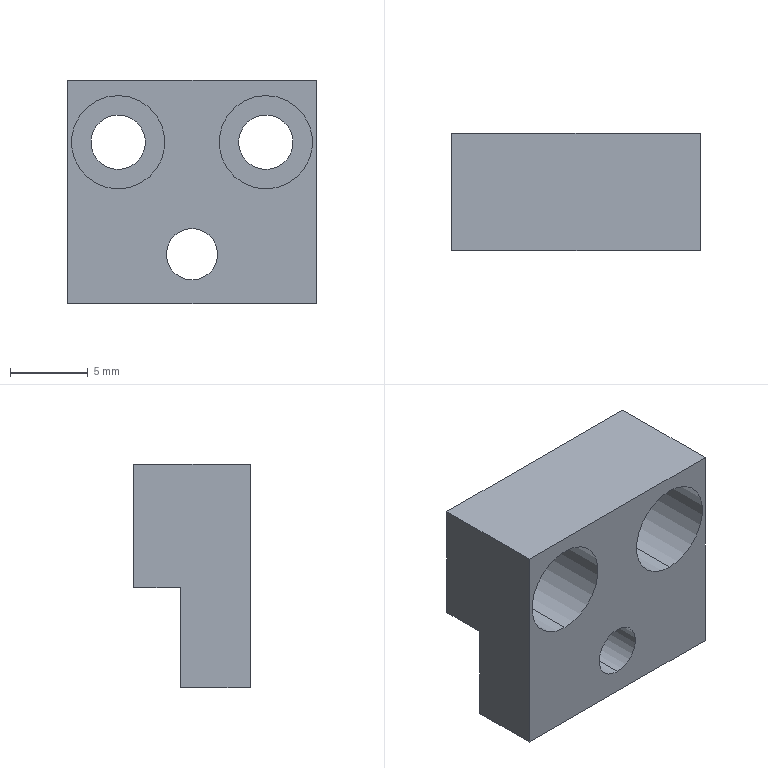Part | NX | 1 solid | 20 faces | box 16 x 7.5 x 14.4 mm | volume 1068 mm3 | plane 10 | cylinder 10 | commonest cylinder face diameters 3.5 x4 6 x4 3.3 x2
STEP:
#1=CARTESIAN_POINT('',(16.39,-66.129,11.453));
#2=VERTEX_POINT('',#1);
#3=CARTESIAN_POINT('',(16.39,-63.129,11.453));
#4=VERTEX_POINT('',#3);
#5=CARTESIAN_POINT('',(16.39,-59.69,11.453));
#6=DIRECTION('',(0.,1.,0.));
#7=VECTOR('',#6,1000.);
#8=LINE('',#5,#7);
#9=EDGE_CURVE('',#2,#4,#8,.T.);
#10=ORIENTED_EDGE('',*,*,#9,.F.);
#11=CARTESIAN_POINT('',(0.3897,-66.129,11.453));
#12=VERTEX_POINT('',#11);
#13=CARTESIAN_POINT('',(13.89,-66.129,11.453));
#14=DIRECTION('',(-1.,0.,0.));
#15=VECTOR('',#14,1000.);
#16=LINE('',#13,#15);
#17=EDGE_CURVE('',#2,#12,#16,.T.);
#18=ORIENTED_EDGE('',*,*,#17,.T.);
#19=CARTESIAN_POINT('',(0.3897,-63.129,11.453));
#20=VERTEX_POINT('',#19);
#21=CARTESIAN_POINT('',(0.3897,-59.69,11.453));
#22=DIRECTION('',(0.,1.,0.));
#23=VECTOR('',#22,1000.);
#24=LINE('',#21,#23);
#25=EDGE_CURVE('',#12,#20,#24,.T.);
#26=ORIENTED_EDGE('',*,*,#25,.T.);
#27=CARTESIAN_POINT('',(13.89,-63.129,11.453));
#28=DIRECTION('',(-1.,0.,0.));
#29=VECTOR('',#28,1000.);
#30=LINE('',#27,#29);
#31=EDGE_CURVE('',#4,#20,#30,.T.);
#32=ORIENTED_EDGE('',*,*,#31,.F.);
#33=EDGE_LOOP('',(#10,#18,#26,#32));
#34=FACE_BOUND('',#33,.T.);
#35=CARTESIAN_POINT('',(13.89,-66.629,11.453));
#36=DIRECTION('',(0.,0.,-1.));
#37=DIRECTION('',(0.,-1.,0.));
#38=AXIS2_PLACEMENT_3D('',#35,#36,#37);
#39=PLANE('',#38);
#40=ADVANCED_FACE('',(#34),#39,.T.);
#41=CARTESIAN_POINT('',(16.39,-66.129,5.003));
#42=VERTEX_POINT('',#41);
#43=CARTESIAN_POINT('',(16.39,-66.129,11.106));
#44=DIRECTION('',(0.,0.,-1.));
#45=VECTOR('',#44,1000.);
#46=LINE('',#43,#45);
#47=EDGE_CURVE('',#2,#42,#46,.T.);
#48=ORIENTED_EDGE('',*,*,#47,.T.);
#49=CARTESIAN_POINT('',(0.3897,-66.129,5.003));
#50=VERTEX_POINT('',#49);
#51=CARTESIAN_POINT('',(13.89,-66.129,5.003));
#52=DIRECTION('',(-1.,0.,0.));
#53=VECTOR('',#52,1000.);
#54=LINE('',#51,#53);
#55=EDGE_CURVE('',#42,#50,#54,.T.);
#56=ORIENTED_EDGE('',*,*,#55,.T.);
#57=CARTESIAN_POINT('',(0.3897,-66.129,11.106));
#58=DIRECTION('',(0.,0.,-1.));
#59=VECTOR('',#58,1000.);
#60=LINE('',#57,#59);
#61=EDGE_CURVE('',#12,#50,#60,.T.);
#62=ORIENTED_EDGE('',*,*,#61,.F.);
#63=ORIENTED_EDGE('',*,*,#17,.F.);
#64=EDGE_LOOP('',(#48,#56,#62,#63));
#65=FACE_BOUND('',#64,.T.);
#66=CARTESIAN_POINT('',(8.39,-66.129,6.553));
#67=VERTEX_POINT('',#66);
#68=CARTESIAN_POINT('',(8.39,-66.129,9.853));
#69=VERTEX_POINT('',#68);
#70=CARTESIAN_POINT('',(8.39,-66.129,8.203));
#71=DIRECTION('',(0.,-1.,0.));
#72=DIRECTION('',(0.,0.,1.));
#73=AXIS2_PLACEMENT_3D('',#70,#71,#72);
#74=CIRCLE('',#73,1.65);
#75=EDGE_CURVE('',#67,#69,#74,.T.);
#76=ORIENTED_EDGE('',*,*,#75,.T.);
#77=CARTESIAN_POINT('',(8.39,-66.129,8.203));
#78=DIRECTION('',(0.,-1.,0.));
#79=DIRECTION('',(0.,0.,1.));
#80=AXIS2_PLACEMENT_3D('',#77,#78,#79);
#81=CIRCLE('',#80,1.65);
#82=EDGE_CURVE('',#69,#67,#81,.T.);
#83=ORIENTED_EDGE('',*,*,#82,.T.);
#84=EDGE_LOOP('',(#76,#83));
#85=FACE_BOUND('',#84,.T.);
#86=CARTESIAN_POINT('',(13.89,-66.129,5.503));
#87=DIRECTION('',(0.,1.,0.));
#88=DIRECTION('',(1.,0.,0.));
#89=AXIS2_PLACEMENT_3D('',#86,#87,#88);
#90=PLANE('',#89);
#91=ADVANCED_FACE('',(#65,#85),#90,.T.);
#92=CARTESIAN_POINT('',(0.3897,-70.629,5.003));
#93=VERTEX_POINT('',#92);
#94=CARTESIAN_POINT('',(16.39,-70.629,5.003));
#95=VERTEX_POINT('',#94);
#96=CARTESIAN_POINT('',(13.89,-70.629,5.003));
#97=DIRECTION('',(1.,0.,0.));
#98=VECTOR('',#97,1000.);
#99=LINE('',#96,#98);
#100=EDGE_CURVE('',#93,#95,#99,.T.);
#101=ORIENTED_EDGE('',*,*,#100,.F.);
#102=CARTESIAN_POINT('',(0.3897,-59.69,5.003));
#103=DIRECTION('',(0.,-1.,0.));
#104=VECTOR('',#103,1000.);
#105=LINE('',#102,#104);
#106=EDGE_CURVE('',#50,#93,#105,.T.);
#107=ORIENTED_EDGE('',*,*,#106,.F.);
#108=ORIENTED_EDGE('',*,*,#55,.F.);
#109=CARTESIAN_POINT('',(16.39,-59.69,5.003));
#110=DIRECTION('',(0.,-1.,0.));
#111=VECTOR('',#110,1000.);
#112=LINE('',#109,#111);
#113=EDGE_CURVE('',#42,#95,#112,.T.);
#114=ORIENTED_EDGE('',*,*,#113,.T.);
#115=EDGE_LOOP('',(#101,#107,#108,#114));
#116=FACE_BOUND('',#115,.T.);
#117=CARTESIAN_POINT('',(13.89,-70.329,5.003));
#118=DIRECTION('',(0.,0.,-1.));
#119=DIRECTION('',(0.,-1.,0.));
#120=AXIS2_PLACEMENT_3D('',#117,#118,#119);
#121=PLANE('',#120);
#122=ADVANCED_FACE('',(#116),#121,.T.);
#123=CARTESIAN_POINT('',(16.39,-70.629,19.403));
#124=VERTEX_POINT('',#123);
#125=CARTESIAN_POINT('',(16.39,-70.629,11.106));
#126=DIRECTION('',(0.,0.,1.));
#127=VECTOR('',#126,1000.);
#128=LINE('',#125,#127);
#129=EDGE_CURVE('',#95,#124,#128,.T.);
#130=ORIENTED_EDGE('',*,*,#129,.T.);
#131=CARTESIAN_POINT('',(0.3897,-70.629,19.403));
#132=VERTEX_POINT('',#131);
#133=CARTESIAN_POINT('',(13.89,-70.629,19.403));
#134=DIRECTION('',(-1.,0.,0.));
#135=VECTOR('',#134,1000.);
#136=LINE('',#133,#135);
#137=EDGE_CURVE('',#124,#132,#136,.T.);
#138=ORIENTED_EDGE('',*,*,#137,.T.);
#139=CARTESIAN_POINT('',(0.3897,-70.629,11.106));
#140=DIRECTION('',(0.,0.,1.));
#141=VECTOR('',#140,1000.);
#142=LINE('',#139,#141);
#143=EDGE_CURVE('',#93,#132,#142,.T.);
#144=ORIENTED_EDGE('',*,*,#143,.F.);
#145=ORIENTED_EDGE('',*,*,#100,.T.);
#146=EDGE_LOOP('',(#130,#138,#144,#145));
#147=FACE_BOUND('',#146,.T.);
#148=CARTESIAN_POINT('',(3.64,-70.629,12.403));
#149=VERTEX_POINT('',#148);
#150=CARTESIAN_POINT('',(3.64,-70.629,18.403));
#151=VERTEX_POINT('',#150);
#152=CARTESIAN_POINT('',(3.64,-70.629,15.403));
#153=DIRECTION('',(0.,-1.,0.));
#154=DIRECTION('',(0.,0.,1.));
#155=AXIS2_PLACEMENT_3D('',#152,#153,#154);
#156=CIRCLE('',#155,3.);
#157=EDGE_CURVE('',#149,#151,#156,.T.);
#158=ORIENTED_EDGE('',*,*,#157,.F.);
#159=CARTESIAN_POINT('',(3.64,-70.629,15.403));
#160=DIRECTION('',(0.,-1.,0.));
#161=DIRECTION('',(0.,0.,1.));
#162=AXIS2_PLACEMENT_3D('',#159,#160,#161);
#163=CIRCLE('',#162,3.);
#164=EDGE_CURVE('',#151,#149,#163,.T.);
#165=ORIENTED_EDGE('',*,*,#164,.F.);
#166=EDGE_LOOP('',(#158,#165));
#167=FACE_BOUND('',#166,.T.);
#168=CARTESIAN_POINT('',(8.39,-70.629,6.553));
#169=VERTEX_POINT('',#168);
#170=CARTESIAN_POINT('',(8.39,-70.629,9.853));
#171=VERTEX_POINT('',#170);
#172=CARTESIAN_POINT('',(8.39,-70.629,8.203));
#173=DIRECTION('',(0.,-1.,0.));
#174=DIRECTION('',(0.,0.,1.));
#175=AXIS2_PLACEMENT_3D('',#172,#173,#174);
#176=CIRCLE('',#175,1.65);
#177=EDGE_CURVE('',#169,#171,#176,.T.);
#178=ORIENTED_EDGE('',*,*,#177,.F.);
#179=CARTESIAN_POINT('',(8.39,-70.629,8.203));
#180=DIRECTION('',(0.,-1.,0.));
#181=DIRECTION('',(0.,0.,1.));
#182=AXIS2_PLACEMENT_3D('',#179,#180,#181);
#183=CIRCLE('',#182,1.65);
#184=EDGE_CURVE('',#171,#169,#183,.T.);
#185=ORIENTED_EDGE('',*,*,#184,.F.);
#186=EDGE_LOOP('',(#178,#185));
#187=FACE_BOUND('',#186,.T.);
#188=CARTESIAN_POINT('',(13.14,-70.629,12.403));
#189=VERTEX_POINT('',#188);
#190=CARTESIAN_POINT('',(13.14,-70.629,18.403));
#191=VERTEX_POINT('',#190);
#192=CARTESIAN_POINT('',(13.14,-70.629,15.403));
#193=DIRECTION('',(0.,-1.,0.));
#194=DIRECTION('',(0.,0.,1.));
#195=AXIS2_PLACEMENT_3D('',#192,#193,#194);
#196=CIRCLE('',#195,3.);
#197=EDGE_CURVE('',#189,#191,#196,.T.);
#198=ORIENTED_EDGE('',*,*,#197,.F.);
#199=CARTESIAN_POINT('',(13.14,-70.629,15.403));
#200=DIRECTION('',(0.,-1.,0.));
#201=DIRECTION('',(0.,0.,1.));
#202=AXIS2_PLACEMENT_3D('',#199,#200,#201);
#203=CIRCLE('',#202,3.);
#204=EDGE_CURVE('',#191,#189,#203,.T.);
#205=ORIENTED_EDGE('',*,*,#204,.F.);
#206=EDGE_LOOP('',(#198,#205));
#207=FACE_BOUND('',#206,.T.);
#208=CARTESIAN_POINT('',(13.89,-70.629,20.403));
#209=DIRECTION('',(0.,-1.,0.));
#210=DIRECTION('',(-1.,0.,0.));
#211=AXIS2_PLACEMENT_3D('',#208,#209,#210);
#212=PLANE('',#211);
#213=ADVANCED_FACE('',(#147,#167,#187,#207),#212,.T.);
#214=CARTESIAN_POINT('',(16.39,-63.129,19.403));
#215=VERTEX_POINT('',#214);
#216=CARTESIAN_POINT('',(16.39,-59.69,19.403));
#217=DIRECTION('',(0.,1.,0.));
#218=VECTOR('',#217,1000.);
#219=LINE('',#216,#218);
#220=EDGE_CURVE('',#124,#215,#219,.T.);
#221=ORIENTED_EDGE('',*,*,#220,.T.);
#222=CARTESIAN_POINT('',(0.3897,-63.129,19.403));
#223=VERTEX_POINT('',#222);
#224=CARTESIAN_POINT('',(13.89,-63.129,19.403));
#225=DIRECTION('',(1.,0.,0.));
#226=VECTOR('',#225,1000.);
#227=LINE('',#224,#226);
#228=EDGE_CURVE('',#223,#215,#227,.T.);
#229=ORIENTED_EDGE('',*,*,#228,.F.);
#230=CARTESIAN_POINT('',(0.3897,-59.69,19.403));
#231=DIRECTION('',(0.,1.,0.));
#232=VECTOR('',#231,1000.);
#233=LINE('',#230,#232);
#234=EDGE_CURVE('',#132,#223,#233,.T.);
#235=ORIENTED_EDGE('',*,*,#234,.F.);
#236=ORIENTED_EDGE('',*,*,#137,.F.);
#237=EDGE_LOOP('',(#221,#229,#235,#236));
#238=FACE_BOUND('',#237,.T.);
#239=CARTESIAN_POINT('',(13.89,-63.129,19.403));
#240=DIRECTION('',(0.,0.,1.));
#241=DIRECTION('',(1.,0.,0.));
#242=AXIS2_PLACEMENT_3D('',#239,#240,#241);
#243=PLANE('',#242);
#244=ADVANCED_FACE('',(#238),#243,.T.);
#245=CARTESIAN_POINT('',(16.39,-63.129,11.106));
#246=DIRECTION('',(0.,0.,-1.));
#247=VECTOR('',#246,1000.);
#248=LINE('',#245,#247);
#249=EDGE_CURVE('',#215,#4,#248,.T.);
#250=ORIENTED_EDGE('',*,*,#249,.T.);
#251=ORIENTED_EDGE('',*,*,#31,.T.);
#252=CARTESIAN_POINT('',(0.3897,-63.129,11.106));
#253=DIRECTION('',(0.,0.,-1.));
#254=VECTOR('',#253,1000.);
#255=LINE('',#252,#254);
#256=EDGE_CURVE('',#223,#20,#255,.T.);
#257=ORIENTED_EDGE('',*,*,#256,.F.);
#258=ORIENTED_EDGE('',*,*,#228,.T.);
#259=EDGE_LOOP('',(#250,#251,#257,#258));
#260=FACE_BOUND('',#259,.T.);
#261=CARTESIAN_POINT('',(13.14,-63.129,13.653));
#262=VERTEX_POINT('',#261);
#263=CARTESIAN_POINT('',(13.14,-63.129,17.153));
#264=VERTEX_POINT('',#263);
#265=CARTESIAN_POINT('',(13.14,-63.129,15.403));
#266=DIRECTION('',(0.,-1.,0.));
#267=DIRECTION('',(0.,0.,1.));
#268=AXIS2_PLACEMENT_3D('',#265,#266,#267);
#269=CIRCLE('',#268,1.75);
#270=EDGE_CURVE('',#262,#264,#269,.T.);
#271=ORIENTED_EDGE('',*,*,#270,.T.);
#272=CARTESIAN_POINT('',(13.14,-63.129,15.403));
#273=DIRECTION('',(0.,-1.,0.));
#274=DIRECTION('',(0.,0.,1.));
#275=AXIS2_PLACEMENT_3D('',#272,#273,#274);
#276=CIRCLE('',#275,1.75);
#277=EDGE_CURVE('',#264,#262,#276,.T.);
#278=ORIENTED_EDGE('',*,*,#277,.T.);
#279=EDGE_LOOP('',(#271,#278));
#280=FACE_BOUND('',#279,.T.);
#281=CARTESIAN_POINT('',(3.64,-63.129,13.653));
#282=VERTEX_POINT('',#281);
#283=CARTESIAN_POINT('',(3.64,-63.129,17.153));
#284=VERTEX_POINT('',#283);
#285=CARTESIAN_POINT('',(3.64,-63.129,15.403));
#286=DIRECTION('',(0.,-1.,0.));
#287=DIRECTION('',(0.,0.,1.));
#288=AXIS2_PLACEMENT_3D('',#285,#286,#287);
#289=CIRCLE('',#288,1.75);
#290=EDGE_CURVE('',#282,#284,#289,.T.);
#291=ORIENTED_EDGE('',*,*,#290,.T.);
#292=CARTESIAN_POINT('',(3.64,-63.129,15.403));
#293=DIRECTION('',(0.,-1.,0.));
#294=DIRECTION('',(0.,0.,1.));
#295=AXIS2_PLACEMENT_3D('',#292,#293,#294);
#296=CIRCLE('',#295,1.75);
#297=EDGE_CURVE('',#284,#282,#296,.T.);
#298=ORIENTED_EDGE('',*,*,#297,.T.);
#299=EDGE_LOOP('',(#291,#298));
#300=FACE_BOUND('',#299,.T.);
#301=CARTESIAN_POINT('',(13.89,-63.129,11.253));
#302=DIRECTION('',(0.,1.,0.));
#303=DIRECTION('',(1.,0.,0.));
#304=AXIS2_PLACEMENT_3D('',#301,#302,#303);
#305=PLANE('',#304);
#306=ADVANCED_FACE('',(#260,#280,#300),#305,.T.);
#307=ORIENTED_EDGE('',*,*,#157,.T.);
#308=CARTESIAN_POINT('',(3.64,-66.129,18.403));
#309=VERTEX_POINT('',#308);
#310=CARTESIAN_POINT('',(3.64,-69.629,18.403));
#311=DIRECTION('',(0.,-1.,0.));
#312=VECTOR('',#311,1000.);
#313=LINE('',#310,#312);
#314=EDGE_CURVE('',#309,#151,#313,.T.);
#315=ORIENTED_EDGE('',*,*,#314,.F.);
#316=CARTESIAN_POINT('',(3.64,-66.129,12.403));
#317=VERTEX_POINT('',#316);
#318=CARTESIAN_POINT('',(3.64,-66.129,15.403));
#319=DIRECTION('',(0.,-1.,0.));
#320=DIRECTION('',(0.,0.,1.));
#321=AXIS2_PLACEMENT_3D('',#318,#319,#320);
#322=CIRCLE('',#321,3.);
#323=EDGE_CURVE('',#317,#309,#322,.T.);
#324=ORIENTED_EDGE('',*,*,#323,.F.);
#325=CARTESIAN_POINT('',(3.64,-69.629,12.403));
#326=DIRECTION('',(0.,-1.,0.));
#327=VECTOR('',#326,1000.);
#328=LINE('',#325,#327);
#329=EDGE_CURVE('',#317,#149,#328,.T.);
#330=ORIENTED_EDGE('',*,*,#329,.T.);
#331=EDGE_LOOP('',(#307,#315,#324,#330));
#332=FACE_BOUND('',#331,.T.);
#333=CARTESIAN_POINT('',(3.64,-69.629,15.403));
#334=DIRECTION('',(0.,-1.,0.));
#335=DIRECTION('',(0.,0.,1.));
#336=AXIS2_PLACEMENT_3D('',#333,#334,#335);
#337=CYLINDRICAL_SURFACE('',#336,3.);
#338=ADVANCED_FACE('',(#332),#337,.F.);
#339=ORIENTED_EDGE('',*,*,#323,.T.);
#340=CARTESIAN_POINT('',(3.64,-66.129,15.403));
#341=DIRECTION('',(0.,-1.,0.));
#342=DIRECTION('',(0.,0.,1.));
#343=AXIS2_PLACEMENT_3D('',#340,#341,#342);
#344=CIRCLE('',#343,3.);
#345=EDGE_CURVE('',#309,#317,#344,.T.);
#346=ORIENTED_EDGE('',*,*,#345,.T.);
#347=EDGE_LOOP('',(#339,#346));
#348=FACE_BOUND('',#347,.T.);
#349=CARTESIAN_POINT('',(3.64,-66.129,13.653));
#350=VERTEX_POINT('',#349);
#351=CARTESIAN_POINT('',(3.64,-66.129,17.153));
#352=VERTEX_POINT('',#351);
#353=CARTESIAN_POINT('',(3.64,-66.129,15.403));
#354=DIRECTION('',(0.,-1.,0.));
#355=DIRECTION('',(0.,0.,1.));
#356=AXIS2_PLACEMENT_3D('',#353,#354,#355);
#357=CIRCLE('',#356,1.75);
#358=EDGE_CURVE('',#350,#352,#357,.T.);
#359=ORIENTED_EDGE('',*,*,#358,.F.);
#360=CARTESIAN_POINT('',(3.64,-66.129,15.403));
#361=DIRECTION('',(0.,-1.,0.));
#362=DIRECTION('',(0.,0.,1.));
#363=AXIS2_PLACEMENT_3D('',#360,#361,#362);
#364=CIRCLE('',#363,1.75);
#365=EDGE_CURVE('',#352,#350,#364,.T.);
#366=ORIENTED_EDGE('',*,*,#365,.F.);
#367=EDGE_LOOP('',(#359,#366));
#368=FACE_BOUND('',#367,.T.);
#369=CARTESIAN_POINT('',(3.64,-66.129,15.403));
#370=DIRECTION('',(0.,-1.,0.));
#371=DIRECTION('',(-1.,0.,0.));
#372=AXIS2_PLACEMENT_3D('',#369,#370,#371);
#373=PLANE('',#372);
#374=ADVANCED_FACE('',(#348,#368),#373,.T.);
#375=ORIENTED_EDGE('',*,*,#358,.T.);
#376=CARTESIAN_POINT('',(3.64,-69.629,17.153));
#377=DIRECTION('',(0.,-1.,0.));
#378=VECTOR('',#377,1000.);
#379=LINE('',#376,#378);
#380=EDGE_CURVE('',#284,#352,#379,.T.);
#381=ORIENTED_EDGE('',*,*,#380,.F.);
#382=ORIENTED_EDGE('',*,*,#290,.F.);
#383=CARTESIAN_POINT('',(3.64,-69.629,13.653));
#384=DIRECTION('',(0.,-1.,0.));
#385=VECTOR('',#384,1000.);
#386=LINE('',#383,#385);
#387=EDGE_CURVE('',#282,#350,#386,.T.);
#388=ORIENTED_EDGE('',*,*,#387,.T.);
#389=EDGE_LOOP('',(#375,#381,#382,#388));
#390=FACE_BOUND('',#389,.T.);
#391=CARTESIAN_POINT('',(3.64,-69.629,15.403));
#392=DIRECTION('',(0.,-1.,0.));
#393=DIRECTION('',(0.,0.,1.));
#394=AXIS2_PLACEMENT_3D('',#391,#392,#393);
#395=CYLINDRICAL_SURFACE('',#394,1.75);
#396=ADVANCED_FACE('',(#390),#395,.F.);
#397=CARTESIAN_POINT('',(13.14,-66.129,13.653));
#398=VERTEX_POINT('',#397);
#399=CARTESIAN_POINT('',(13.14,-66.129,17.153));
#400=VERTEX_POINT('',#399);
#401=CARTESIAN_POINT('',(13.14,-66.129,15.403));
#402=DIRECTION('',(0.,-1.,0.));
#403=DIRECTION('',(0.,0.,1.));
#404=AXIS2_PLACEMENT_3D('',#401,#402,#403);
#405=CIRCLE('',#404,1.75);
#406=EDGE_CURVE('',#398,#400,#405,.T.);
#407=ORIENTED_EDGE('',*,*,#406,.T.);
#408=CARTESIAN_POINT('',(13.14,-69.629,17.153));
#409=DIRECTION('',(0.,-1.,0.));
#410=VECTOR('',#409,1000.);
#411=LINE('',#408,#410);
#412=EDGE_CURVE('',#264,#400,#411,.T.);
#413=ORIENTED_EDGE('',*,*,#412,.F.);
#414=ORIENTED_EDGE('',*,*,#270,.F.);
#415=CARTESIAN_POINT('',(13.14,-69.629,13.653));
#416=DIRECTION('',(0.,-1.,0.));
#417=VECTOR('',#416,1000.);
#418=LINE('',#415,#417);
#419=EDGE_CURVE('',#262,#398,#418,.T.);
#420=ORIENTED_EDGE('',*,*,#419,.T.);
#421=EDGE_LOOP('',(#407,#413,#414,#420));
#422=FACE_BOUND('',#421,.T.);
#423=CARTESIAN_POINT('',(13.14,-69.629,15.403));
#424=DIRECTION('',(0.,-1.,0.));
#425=DIRECTION('',(0.,0.,1.));
#426=AXIS2_PLACEMENT_3D('',#423,#424,#425);
#427=CYLINDRICAL_SURFACE('',#426,1.75);
#428=ADVANCED_FACE('',(#422),#427,.F.);
#429=CARTESIAN_POINT('',(13.14,-66.129,12.403));
#430=VERTEX_POINT('',#429);
#431=CARTESIAN_POINT('',(13.14,-66.129,18.403));
#432=VERTEX_POINT('',#431);
#433=CARTESIAN_POINT('',(13.14,-66.129,15.403));
#434=DIRECTION('',(0.,-1.,0.));
#435=DIRECTION('',(0.,0.,1.));
#436=AXIS2_PLACEMENT_3D('',#433,#434,#435);
#437=CIRCLE('',#436,3.);
#438=EDGE_CURVE('',#430,#432,#437,.T.);
#439=ORIENTED_EDGE('',*,*,#438,.T.);
#440=CARTESIAN_POINT('',(13.14,-66.129,15.403));
#441=DIRECTION('',(0.,-1.,0.));
#442=DIRECTION('',(0.,0.,1.));
#443=AXIS2_PLACEMENT_3D('',#440,#441,#442);
#444=CIRCLE('',#443,3.);
#445=EDGE_CURVE('',#432,#430,#444,.T.);
#446=ORIENTED_EDGE('',*,*,#445,.T.);
#447=EDGE_LOOP('',(#439,#446));
#448=FACE_BOUND('',#447,.T.);
#449=ORIENTED_EDGE('',*,*,#406,.F.);
#450=CARTESIAN_POINT('',(13.14,-66.129,15.403));
#451=DIRECTION('',(0.,-1.,0.));
#452=DIRECTION('',(0.,0.,1.));
#453=AXIS2_PLACEMENT_3D('',#450,#451,#452);
#454=CIRCLE('',#453,1.75);
#455=EDGE_CURVE('',#400,#398,#454,.T.);
#456=ORIENTED_EDGE('',*,*,#455,.F.);
#457=EDGE_LOOP('',(#449,#456));
#458=FACE_BOUND('',#457,.T.);
#459=CARTESIAN_POINT('',(13.14,-66.129,15.403));
#460=DIRECTION('',(0.,-1.,0.));
#461=DIRECTION('',(-1.,0.,0.));
#462=AXIS2_PLACEMENT_3D('',#459,#460,#461);
#463=PLANE('',#462);
#464=ADVANCED_FACE('',(#448,#458),#463,.T.);
#465=ORIENTED_EDGE('',*,*,#197,.T.);
#466=CARTESIAN_POINT('',(13.14,-69.629,18.403));
#467=DIRECTION('',(0.,-1.,0.));
#468=VECTOR('',#467,1000.);
#469=LINE('',#466,#468);
#470=EDGE_CURVE('',#432,#191,#469,.T.);
#471=ORIENTED_EDGE('',*,*,#470,.F.);
#472=ORIENTED_EDGE('',*,*,#438,.F.);
#473=CARTESIAN_POINT('',(13.14,-69.629,12.403));
#474=DIRECTION('',(0.,-1.,0.));
#475=VECTOR('',#474,1000.);
#476=LINE('',#473,#475);
#477=EDGE_CURVE('',#430,#189,#476,.T.);
#478=ORIENTED_EDGE('',*,*,#477,.T.);
#479=EDGE_LOOP('',(#465,#471,#472,#478));
#480=FACE_BOUND('',#479,.T.);
#481=CARTESIAN_POINT('',(13.14,-69.629,15.403));
#482=DIRECTION('',(0.,-1.,0.));
#483=DIRECTION('',(0.,0.,1.));
#484=AXIS2_PLACEMENT_3D('',#481,#482,#483);
#485=CYLINDRICAL_SURFACE('',#484,3.);
#486=ADVANCED_FACE('',(#480),#485,.F.);
#487=ORIENTED_EDGE('',*,*,#177,.T.);
#488=CARTESIAN_POINT('',(8.39,-69.629,9.853));
#489=DIRECTION('',(0.,-1.,0.));
#490=VECTOR('',#489,1000.);
#491=LINE('',#488,#490);
#492=EDGE_CURVE('',#69,#171,#491,.T.);
#493=ORIENTED_EDGE('',*,*,#492,.F.);
#494=ORIENTED_EDGE('',*,*,#75,.F.);
#495=CARTESIAN_POINT('',(8.39,-69.629,6.553));
#496=DIRECTION('',(0.,-1.,0.));
#497=VECTOR('',#496,1000.);
#498=LINE('',#495,#497);
#499=EDGE_CURVE('',#67,#169,#498,.T.);
#500=ORIENTED_EDGE('',*,*,#499,.T.);
#501=EDGE_LOOP('',(#487,#493,#494,#500));
#502=FACE_BOUND('',#501,.T.);
#503=CARTESIAN_POINT('',(8.39,-69.629,8.203));
#504=DIRECTION('',(0.,-1.,0.));
#505=DIRECTION('',(0.,0.,1.));
#506=AXIS2_PLACEMENT_3D('',#503,#504,#505);
#507=CYLINDRICAL_SURFACE('',#506,1.65);
#508=ADVANCED_FACE('',(#502),#507,.F.);
#509=ORIENTED_EDGE('',*,*,#492,.T.);
#510=ORIENTED_EDGE('',*,*,#184,.T.);
#511=ORIENTED_EDGE('',*,*,#499,.F.);
#512=ORIENTED_EDGE('',*,*,#82,.F.);
#513=EDGE_LOOP('',(#509,#510,#511,#512));
#514=FACE_BOUND('',#513,.T.);
#515=CARTESIAN_POINT('',(8.39,-69.629,8.203));
#516=DIRECTION('',(0.,-1.,0.));
#517=DIRECTION('',(0.,0.,1.));
#518=AXIS2_PLACEMENT_3D('',#515,#516,#517);
#519=CYLINDRICAL_SURFACE('',#518,1.65);
#520=ADVANCED_FACE('',(#514),#519,.F.);
#521=ORIENTED_EDGE('',*,*,#314,.T.);
#522=ORIENTED_EDGE('',*,*,#164,.T.);
#523=ORIENTED_EDGE('',*,*,#329,.F.);
#524=ORIENTED_EDGE('',*,*,#345,.F.);
#525=EDGE_LOOP('',(#521,#522,#523,#524));
#526=FACE_BOUND('',#525,.T.);
#527=CARTESIAN_POINT('',(3.64,-69.629,15.403));
#528=DIRECTION('',(0.,-1.,0.));
#529=DIRECTION('',(0.,0.,1.));
#530=AXIS2_PLACEMENT_3D('',#527,#528,#529);
#531=CYLINDRICAL_SURFACE('',#530,3.);
#532=ADVANCED_FACE('',(#526),#531,.F.);
#533=ORIENTED_EDGE('',*,*,#470,.T.);
#534=ORIENTED_EDGE('',*,*,#204,.T.);
#535=ORIENTED_EDGE('',*,*,#477,.F.);
#536=ORIENTED_EDGE('',*,*,#445,.F.);
#537=EDGE_LOOP('',(#533,#534,#535,#536));
#538=FACE_BOUND('',#537,.T.);
#539=CARTESIAN_POINT('',(13.14,-69.629,15.403));
#540=DIRECTION('',(0.,-1.,0.));
#541=DIRECTION('',(0.,0.,1.));
#542=AXIS2_PLACEMENT_3D('',#539,#540,#541);
#543=CYLINDRICAL_SURFACE('',#542,3.);
#544=ADVANCED_FACE('',(#538),#543,.F.);
#545=ORIENTED_EDGE('',*,*,#412,.T.);
#546=ORIENTED_EDGE('',*,*,#455,.T.);
#547=ORIENTED_EDGE('',*,*,#419,.F.);
#548=ORIENTED_EDGE('',*,*,#277,.F.);
#549=EDGE_LOOP('',(#545,#546,#547,#548));
#550=FACE_BOUND('',#549,.T.);
#551=CARTESIAN_POINT('',(13.14,-69.629,15.403));
#552=DIRECTION('',(0.,-1.,0.));
#553=DIRECTION('',(0.,0.,1.));
#554=AXIS2_PLACEMENT_3D('',#551,#552,#553);
#555=CYLINDRICAL_SURFACE('',#554,1.75);
#556=ADVANCED_FACE('',(#550),#555,.F.);
#557=ORIENTED_EDGE('',*,*,#380,.T.);
#558=ORIENTED_EDGE('',*,*,#365,.T.);
#559=ORIENTED_EDGE('',*,*,#387,.F.);
#560=ORIENTED_EDGE('',*,*,#297,.F.);
#561=EDGE_LOOP('',(#557,#558,#559,#560));
#562=FACE_BOUND('',#561,.T.);
#563=CARTESIAN_POINT('',(3.64,-69.629,15.403));
#564=DIRECTION('',(0.,-1.,0.));
#565=DIRECTION('',(0.,0.,1.));
#566=AXIS2_PLACEMENT_3D('',#563,#564,#565);
#567=CYLINDRICAL_SURFACE('',#566,1.75);
#568=ADVANCED_FACE('',(#562),#567,.F.);
#569=ORIENTED_EDGE('',*,*,#61,.T.);
#570=ORIENTED_EDGE('',*,*,#106,.T.);
#571=ORIENTED_EDGE('',*,*,#143,.T.);
#572=ORIENTED_EDGE('',*,*,#234,.T.);
#573=ORIENTED_EDGE('',*,*,#256,.T.);
#574=ORIENTED_EDGE('',*,*,#25,.F.);
#575=EDGE_LOOP('',(#569,#570,#571,#572,#573,#574));
#576=FACE_BOUND('',#575,.T.);
#577=CARTESIAN_POINT('',(0.3897,-59.69,11.106));
#578=DIRECTION('',(1.,0.,0.));
#579=DIRECTION('',(0.,-1.,0.));
#580=AXIS2_PLACEMENT_3D('',#577,#578,#579);
#581=PLANE('',#580);
#582=ADVANCED_FACE('',(#576),#581,.F.);
#583=ORIENTED_EDGE('',*,*,#9,.T.);
#584=ORIENTED_EDGE('',*,*,#249,.F.);
#585=ORIENTED_EDGE('',*,*,#220,.F.);
#586=ORIENTED_EDGE('',*,*,#129,.F.);
#587=ORIENTED_EDGE('',*,*,#113,.F.);
#588=ORIENTED_EDGE('',*,*,#47,.F.);
#589=EDGE_LOOP('',(#583,#584,#585,#586,#587,#588));
#590=FACE_BOUND('',#589,.T.);
#591=CARTESIAN_POINT('',(16.39,-59.69,11.106));
#592=DIRECTION('',(1.,0.,0.));
#593=DIRECTION('',(0.,-1.,0.));
#594=AXIS2_PLACEMENT_3D('',#591,#592,#593);
#595=PLANE('',#594);
#596=ADVANCED_FACE('',(#590),#595,.T.);
#597=CLOSED_SHELL('',(#40,#91,#122,#213,#244,#306,#338,#374,#396,#428,#464,#486,#508,#520,#532,#544,#556,#568,#582,#596));
#598=MANIFOLD_SOLID_BREP('',#597);
#599=(LENGTH_UNIT()NAMED_UNIT(*)SI_UNIT(.MILLI.,.METRE.));
#600=UNCERTAINTY_MEASURE_WITH_UNIT(LENGTH_MEASURE(0.00001),#599,'','');
#601=(NAMED_UNIT(*)PLANE_ANGLE_UNIT()SI_UNIT($,.RADIAN.));
#602=(NAMED_UNIT(*)SI_UNIT($,.STERADIAN.)SOLID_ANGLE_UNIT());
#603=(GEOMETRIC_REPRESENTATION_CONTEXT(3)GLOBAL_UNCERTAINTY_ASSIGNED_CONTEXT((#600))GLOBAL_UNIT_ASSIGNED_CONTEXT((#599,#601,#602))REPRESENTATION_CONTEXT('',''));
#604=ADVANCED_BREP_SHAPE_REPRESENTATION('',(#598),#603);